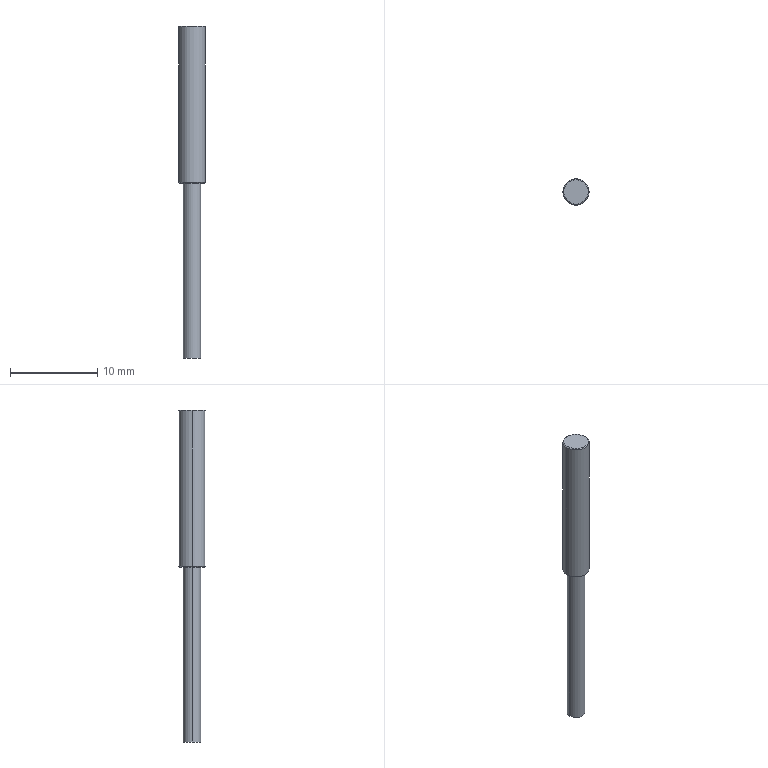Part | STEP file | E32-C42S 1M | 1 solid | 11 faces | box 3 x 3 x 38 mm | volume 189.974 mm3 | cylinder 4 | cone 4 | plane 3 | commonest cylinder face diameters 2 x2 3 x2
STEP:
#1=CARTESIAN_POINT('',(-1.,0.,-20.));
#2=VERTEX_POINT('',#1);
#3=CARTESIAN_POINT('',(1.,0.,-20.));
#4=VERTEX_POINT('',#3);
#5=CARTESIAN_POINT('',(0.,0.,-20.));
#6=DIRECTION('',(0.,0.,-1.));
#7=DIRECTION('',(-1.,0.,0.));
#8=AXIS2_PLACEMENT_3D('',#5,#6,#7);
#9=CIRCLE('',#8,1.);
#10=EDGE_CURVE('',#2,#4,#9,.T.);
#11=ORIENTED_EDGE('',*,*,#10,.F.);
#12=CARTESIAN_POINT('',(-1.,0.,0.));
#13=VERTEX_POINT('',#12);
#14=CARTESIAN_POINT('',(-1.,0.,-20.));
#15=DIRECTION('',(0.,0.,1.));
#16=VECTOR('',#15,1000.);
#17=LINE('',#14,#16);
#18=EDGE_CURVE('',#2,#13,#17,.T.);
#19=ORIENTED_EDGE('',*,*,#18,.T.);
#20=CARTESIAN_POINT('',(1.,0.,0.));
#21=VERTEX_POINT('',#20);
#22=CARTESIAN_POINT('',(0.,0.,0.));
#23=DIRECTION('',(0.,0.,-1.));
#24=DIRECTION('',(1.,0.,0.));
#25=AXIS2_PLACEMENT_3D('',#22,#23,#24);
#26=CIRCLE('',#25,1.);
#27=EDGE_CURVE('',#13,#21,#26,.T.);
#28=ORIENTED_EDGE('',*,*,#27,.T.);
#29=CARTESIAN_POINT('',(1.,0.,-20.));
#30=DIRECTION('',(0.,0.,1.));
#31=VECTOR('',#30,1000.);
#32=LINE('',#29,#31);
#33=EDGE_CURVE('',#4,#21,#32,.T.);
#34=ORIENTED_EDGE('',*,*,#33,.F.);
#35=EDGE_LOOP('',(#11,#19,#28,#34));
#36=FACE_OUTER_BOUND('',#35,.T.);
#37=CARTESIAN_POINT('',(0.,0.,-20.));
#38=DIRECTION('',(0.,0.,1.));
#39=DIRECTION('',(1.,0.,0.));
#40=AXIS2_PLACEMENT_3D('',#37,#38,#39);
#41=CYLINDRICAL_SURFACE('',#40,1.);
#42=ADVANCED_FACE('',(#36),#41,.T.);
#43=CARTESIAN_POINT('',(1.4,0.,18.));
#44=VERTEX_POINT('',#43);
#45=CARTESIAN_POINT('',(-1.4,0.,18.));
#46=VERTEX_POINT('',#45);
#47=CARTESIAN_POINT('',(0.,0.,18.));
#48=DIRECTION('',(0.,0.,1.));
#49=DIRECTION('',(1.,0.,0.));
#50=AXIS2_PLACEMENT_3D('',#47,#48,#49);
#51=CIRCLE('',#50,1.4);
#52=EDGE_CURVE('',#44,#46,#51,.T.);
#53=ORIENTED_EDGE('',*,*,#52,.F.);
#54=CARTESIAN_POINT('',(1.5,0.,17.9));
#55=VERTEX_POINT('',#54);
#56=CARTESIAN_POINT('',(1.4,0.,18.));
#57=DIRECTION('',(0.7071,0.,-0.7071));
#58=VECTOR('',#57,1000.);
#59=LINE('',#56,#58);
#60=EDGE_CURVE('',#44,#55,#59,.T.);
#61=ORIENTED_EDGE('',*,*,#60,.T.);
#62=CARTESIAN_POINT('',(-1.5,0.,17.9));
#63=VERTEX_POINT('',#62);
#64=CARTESIAN_POINT('',(0.,0.,17.9));
#65=DIRECTION('',(0.,0.,-1.));
#66=DIRECTION('',(1.,0.,0.));
#67=AXIS2_PLACEMENT_3D('',#64,#65,#66);
#68=CIRCLE('',#67,1.5);
#69=EDGE_CURVE('',#63,#55,#68,.T.);
#70=ORIENTED_EDGE('',*,*,#69,.F.);
#71=CARTESIAN_POINT('',(-1.4,0.,18.));
#72=DIRECTION('',(-0.7071,0.,-0.7071));
#73=VECTOR('',#72,1000.);
#74=LINE('',#71,#73);
#75=EDGE_CURVE('',#46,#63,#74,.T.);
#76=ORIENTED_EDGE('',*,*,#75,.F.);
#77=EDGE_LOOP('',(#53,#61,#70,#76));
#78=FACE_OUTER_BOUND('',#77,.T.);
#79=CARTESIAN_POINT('',(0.,0.,18.));
#80=DIRECTION('',(0.,0.,-1.));
#81=DIRECTION('',(-1.,0.,0.));
#82=AXIS2_PLACEMENT_3D('',#79,#80,#81);
#83=CONICAL_SURFACE('',#82,1.4,0.7854);
#84=ADVANCED_FACE('',(#78),#83,.T.);
#85=CARTESIAN_POINT('',(-1.4,0.,0.));
#86=VERTEX_POINT('',#85);
#87=CARTESIAN_POINT('',(1.4,0.,0.));
#88=VERTEX_POINT('',#87);
#89=CARTESIAN_POINT('',(0.,0.,0.));
#90=DIRECTION('',(0.,0.,-1.));
#91=DIRECTION('',(1.,0.,0.));
#92=AXIS2_PLACEMENT_3D('',#89,#90,#91);
#93=CIRCLE('',#92,1.4);
#94=EDGE_CURVE('',#86,#88,#93,.T.);
#95=ORIENTED_EDGE('',*,*,#94,.F.);
#96=CARTESIAN_POINT('',(-1.5,0.,0.1));
#97=VERTEX_POINT('',#96);
#98=CARTESIAN_POINT('',(-1.5,0.,0.1));
#99=DIRECTION('',(-0.7071,0.,0.7071));
#100=VECTOR('',#99,1000.);
#101=LINE('',#98,#100);
#102=EDGE_CURVE('',#86,#97,#101,.T.);
#103=ORIENTED_EDGE('',*,*,#102,.T.);
#104=CARTESIAN_POINT('',(1.5,0.,0.1));
#105=VERTEX_POINT('',#104);
#106=CARTESIAN_POINT('',(0.,0.,0.1));
#107=DIRECTION('',(0.,0.,1.));
#108=DIRECTION('',(1.,0.,0.));
#109=AXIS2_PLACEMENT_3D('',#106,#107,#108);
#110=CIRCLE('',#109,1.5);
#111=EDGE_CURVE('',#105,#97,#110,.T.);
#112=ORIENTED_EDGE('',*,*,#111,.F.);
#113=CARTESIAN_POINT('',(1.5,0.,0.1));
#114=DIRECTION('',(0.7071,0.,0.7071));
#115=VECTOR('',#114,1000.);
#116=LINE('',#113,#115);
#117=EDGE_CURVE('',#88,#105,#116,.T.);
#118=ORIENTED_EDGE('',*,*,#117,.F.);
#119=EDGE_LOOP('',(#95,#103,#112,#118));
#120=FACE_OUTER_BOUND('',#119,.T.);
#121=CARTESIAN_POINT('',(0.,0.,0.1));
#122=DIRECTION('',(0.,0.,1.));
#123=DIRECTION('',(1.,0.,0.));
#124=AXIS2_PLACEMENT_3D('',#121,#122,#123);
#125=CONICAL_SURFACE('',#124,1.5,0.7854);
#126=ADVANCED_FACE('',(#120),#125,.T.);
#127=ORIENTED_EDGE('',*,*,#69,.T.);
#128=CARTESIAN_POINT('',(1.5,0.,18.));
#129=DIRECTION('',(0.,0.,-1.));
#130=VECTOR('',#129,1000.);
#131=LINE('',#128,#130);
#132=EDGE_CURVE('',#55,#105,#131,.T.);
#133=ORIENTED_EDGE('',*,*,#132,.T.);
#134=ORIENTED_EDGE('',*,*,#111,.T.);
#135=CARTESIAN_POINT('',(-1.5,0.,18.));
#136=DIRECTION('',(0.,0.,-1.));
#137=VECTOR('',#136,1000.);
#138=LINE('',#135,#137);
#139=EDGE_CURVE('',#63,#97,#138,.T.);
#140=ORIENTED_EDGE('',*,*,#139,.F.);
#141=EDGE_LOOP('',(#127,#133,#134,#140));
#142=FACE_OUTER_BOUND('',#141,.T.);
#143=CARTESIAN_POINT('',(0.,0.,18.));
#144=DIRECTION('',(0.,0.,-1.));
#145=DIRECTION('',(-1.,0.,0.));
#146=AXIS2_PLACEMENT_3D('',#143,#144,#145);
#147=CYLINDRICAL_SURFACE('',#146,1.5);
#148=ADVANCED_FACE('',(#142),#147,.T.);
#149=CARTESIAN_POINT('',(0.,0.,0.));
#150=DIRECTION('',(0.,0.,-1.));
#151=DIRECTION('',(1.,0.,0.));
#152=AXIS2_PLACEMENT_3D('',#149,#150,#151);
#153=CIRCLE('',#152,1.4);
#154=EDGE_CURVE('',#88,#86,#153,.T.);
#155=ORIENTED_EDGE('',*,*,#154,.T.);
#156=ORIENTED_EDGE('',*,*,#94,.T.);
#157=EDGE_LOOP('',(#155,#156));
#158=FACE_OUTER_BOUND('',#157,.T.);
#159=CARTESIAN_POINT('',(0.,0.,0.));
#160=DIRECTION('',(0.,0.,-1.));
#161=DIRECTION('',(1.,0.,0.));
#162=AXIS2_PLACEMENT_3D('',#159,#160,#161);
#163=CIRCLE('',#162,1.);
#164=EDGE_CURVE('',#21,#13,#163,.T.);
#165=ORIENTED_EDGE('',*,*,#164,.F.);
#166=ORIENTED_EDGE('',*,*,#27,.F.);
#167=EDGE_LOOP('',(#165,#166));
#168=FACE_BOUND('',#167,.T.);
#169=CARTESIAN_POINT('',(0.,0.,0.));
#170=DIRECTION('',(0.,0.,1.));
#171=DIRECTION('',(1.,0.,0.));
#172=AXIS2_PLACEMENT_3D('',#169,#170,#171);
#173=PLANE('',#172);
#174=ADVANCED_FACE('',(#158,#168),#173,.F.);
#175=ORIENTED_EDGE('',*,*,#132,.F.);
#176=CARTESIAN_POINT('',(0.,0.,17.9));
#177=DIRECTION('',(0.,0.,-1.));
#178=DIRECTION('',(1.,0.,0.));
#179=AXIS2_PLACEMENT_3D('',#176,#177,#178);
#180=CIRCLE('',#179,1.5);
#181=EDGE_CURVE('',#55,#63,#180,.T.);
#182=ORIENTED_EDGE('',*,*,#181,.T.);
#183=ORIENTED_EDGE('',*,*,#139,.T.);
#184=CARTESIAN_POINT('',(0.,0.,0.1));
#185=DIRECTION('',(0.,0.,1.));
#186=DIRECTION('',(1.,0.,0.));
#187=AXIS2_PLACEMENT_3D('',#184,#185,#186);
#188=CIRCLE('',#187,1.5);
#189=EDGE_CURVE('',#97,#105,#188,.T.);
#190=ORIENTED_EDGE('',*,*,#189,.T.);
#191=EDGE_LOOP('',(#175,#182,#183,#190));
#192=FACE_OUTER_BOUND('',#191,.T.);
#193=CARTESIAN_POINT('',(0.,0.,18.));
#194=DIRECTION('',(0.,0.,-1.));
#195=DIRECTION('',(-1.,0.,0.));
#196=AXIS2_PLACEMENT_3D('',#193,#194,#195);
#197=CYLINDRICAL_SURFACE('',#196,1.5);
#198=ADVANCED_FACE('',(#192),#197,.T.);
#199=CARTESIAN_POINT('',(0.,0.,18.));
#200=DIRECTION('',(0.,0.,1.));
#201=DIRECTION('',(1.,0.,0.));
#202=AXIS2_PLACEMENT_3D('',#199,#200,#201);
#203=CIRCLE('',#202,1.4);
#204=EDGE_CURVE('',#46,#44,#203,.T.);
#205=ORIENTED_EDGE('',*,*,#204,.T.);
#206=ORIENTED_EDGE('',*,*,#52,.T.);
#207=EDGE_LOOP('',(#205,#206));
#208=FACE_OUTER_BOUND('',#207,.T.);
#209=CARTESIAN_POINT('',(0.,0.,18.));
#210=DIRECTION('',(0.,0.,1.));
#211=DIRECTION('',(1.,0.,0.));
#212=AXIS2_PLACEMENT_3D('',#209,#210,#211);
#213=PLANE('',#212);
#214=ADVANCED_FACE('',(#208),#213,.T.);
#215=ORIENTED_EDGE('',*,*,#102,.F.);
#216=ORIENTED_EDGE('',*,*,#154,.F.);
#217=ORIENTED_EDGE('',*,*,#117,.T.);
#218=ORIENTED_EDGE('',*,*,#189,.F.);
#219=EDGE_LOOP('',(#215,#216,#217,#218));
#220=FACE_OUTER_BOUND('',#219,.T.);
#221=CARTESIAN_POINT('',(0.,0.,0.1));
#222=DIRECTION('',(0.,0.,1.));
#223=DIRECTION('',(1.,0.,0.));
#224=AXIS2_PLACEMENT_3D('',#221,#222,#223);
#225=CONICAL_SURFACE('',#224,1.5,0.7854);
#226=ADVANCED_FACE('',(#220),#225,.T.);
#227=ORIENTED_EDGE('',*,*,#60,.F.);
#228=ORIENTED_EDGE('',*,*,#204,.F.);
#229=ORIENTED_EDGE('',*,*,#75,.T.);
#230=ORIENTED_EDGE('',*,*,#181,.F.);
#231=EDGE_LOOP('',(#227,#228,#229,#230));
#232=FACE_OUTER_BOUND('',#231,.T.);
#233=CARTESIAN_POINT('',(0.,0.,18.));
#234=DIRECTION('',(0.,0.,-1.));
#235=DIRECTION('',(-1.,0.,0.));
#236=AXIS2_PLACEMENT_3D('',#233,#234,#235);
#237=CONICAL_SURFACE('',#236,1.4,0.7854);
#238=ADVANCED_FACE('',(#232),#237,.T.);
#239=ORIENTED_EDGE('',*,*,#18,.F.);
#240=CARTESIAN_POINT('',(0.,0.,-20.));
#241=DIRECTION('',(0.,0.,-1.));
#242=DIRECTION('',(-1.,0.,0.));
#243=AXIS2_PLACEMENT_3D('',#240,#241,#242);
#244=CIRCLE('',#243,1.);
#245=EDGE_CURVE('',#4,#2,#244,.T.);
#246=ORIENTED_EDGE('',*,*,#245,.F.);
#247=ORIENTED_EDGE('',*,*,#33,.T.);
#248=ORIENTED_EDGE('',*,*,#164,.T.);
#249=EDGE_LOOP('',(#239,#246,#247,#248));
#250=FACE_OUTER_BOUND('',#249,.T.);
#251=CARTESIAN_POINT('',(0.,0.,-20.));
#252=DIRECTION('',(0.,0.,1.));
#253=DIRECTION('',(1.,0.,0.));
#254=AXIS2_PLACEMENT_3D('',#251,#252,#253);
#255=CYLINDRICAL_SURFACE('',#254,1.);
#256=ADVANCED_FACE('',(#250),#255,.T.);
#257=ORIENTED_EDGE('',*,*,#245,.T.);
#258=ORIENTED_EDGE('',*,*,#10,.T.);
#259=EDGE_LOOP('',(#257,#258));
#260=FACE_OUTER_BOUND('',#259,.T.);
#261=CARTESIAN_POINT('',(0.,0.,-20.));
#262=DIRECTION('',(0.,0.,-1.));
#263=DIRECTION('',(-1.,0.,0.));
#264=AXIS2_PLACEMENT_3D('',#261,#262,#263);
#265=PLANE('',#264);
#266=ADVANCED_FACE('',(#260),#265,.T.);
#267=CLOSED_SHELL('',(#42,#84,#126,#148,#174,#198,#214,#226,#238,#256,#266));
#268=MANIFOLD_SOLID_BREP('',#267);
#269=CARTESIAN_POINT('',(0.,0.,0.));
#270=DIRECTION('',(0.,0.,1.));
#271=DIRECTION('',(1.,0.,0.));
#272=AXIS2_PLACEMENT_3D('',#269,#270,#271);
#273=(LENGTH_UNIT()NAMED_UNIT(*)SI_UNIT(.MILLI.,.METRE.));
#274=UNCERTAINTY_MEASURE_WITH_UNIT(LENGTH_MEASURE(0.00001),#273,'','');
#275=(NAMED_UNIT(*)PLANE_ANGLE_UNIT()SI_UNIT($,.RADIAN.));
#276=(NAMED_UNIT(*)SI_UNIT($,.STERADIAN.)SOLID_ANGLE_UNIT());
#277=(GEOMETRIC_REPRESENTATION_CONTEXT(3)GLOBAL_UNCERTAINTY_ASSIGNED_CONTEXT((#274))GLOBAL_UNIT_ASSIGNED_CONTEXT((#273,#275,#276))REPRESENTATION_CONTEXT('',''));
#278=ADVANCED_BREP_SHAPE_REPRESENTATION('',(#268,#272),#277);